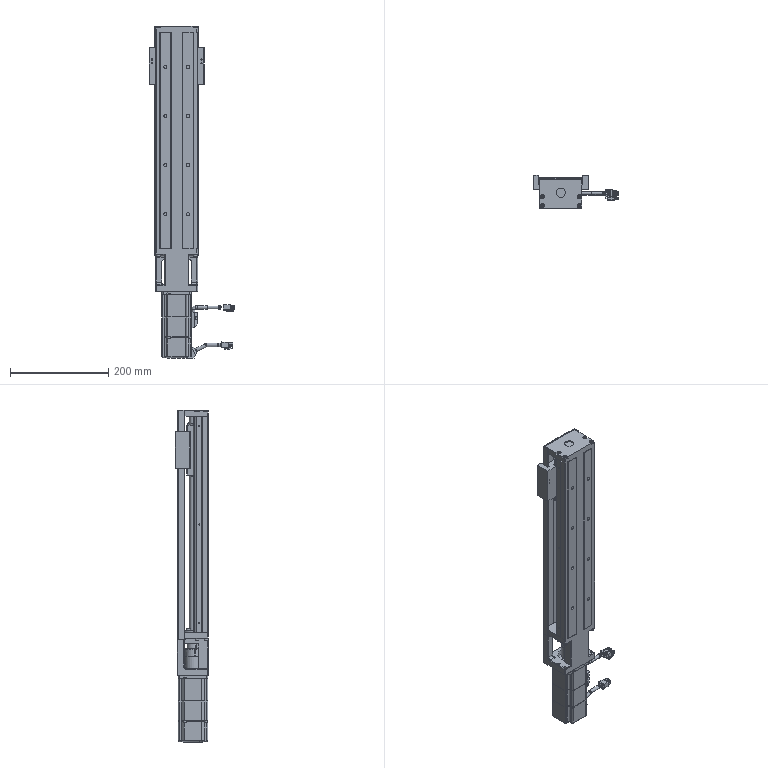Part | NX | 13 solids | 1365 faces | box 174.3 x 68 x 675.5 mm | volume 1844856 mm3 | plane 946 | cylinder 347 | cone 40 | spline 32 | commonest cylinder face diameters 4 x50 3 x31 8 x31 6 x30 0.6 x18 6.5 x18